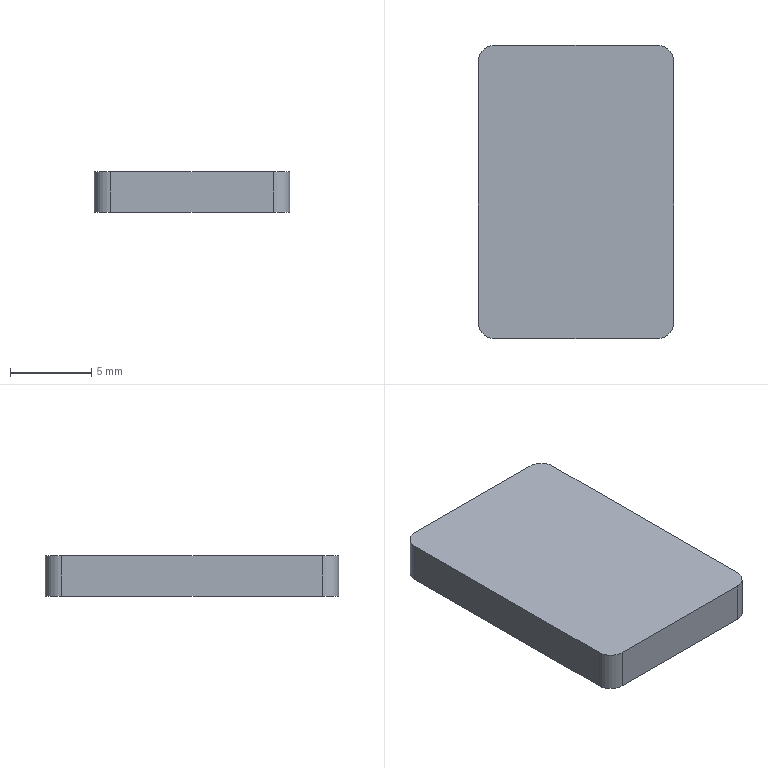Part | STEP file | lll_id938_x_t | 1 solid | 10 faces | box 12 x 18 x 2.5 mm | volume 537.854 mm3 | plane 6 | cylinder 4 | commonest cylinder face diameters 2 x4
STEP:
#1=CARTESIAN_POINT('',(498.87,-355.5,0.));
#2=VERTEX_POINT('',#1);
#3=CARTESIAN_POINT('',(498.87,-339.5,0.));
#4=VERTEX_POINT('',#3);
#5=CARTESIAN_POINT('',(498.87,-355.5,0.));
#6=DIRECTION('',(0.,1.,0.));
#7=VECTOR('',#6,1.);
#8=LINE('',#5,#7);
#9=EDGE_CURVE('',#2,#4,#8,.T.);
#10=ORIENTED_EDGE('',*,*,#9,.T.);
#11=CARTESIAN_POINT('',(498.87,-339.5,2.5));
#12=VERTEX_POINT('',#11);
#13=CARTESIAN_POINT('',(498.87,-339.5,2.5));
#14=DIRECTION('',(0.,0.,-1.));
#15=VECTOR('',#14,1.);
#16=LINE('',#13,#15);
#17=EDGE_CURVE('',#12,#4,#16,.T.);
#18=ORIENTED_EDGE('',*,*,#17,.F.);
#19=CARTESIAN_POINT('',(498.87,-355.5,2.5));
#20=VERTEX_POINT('',#19);
#21=CARTESIAN_POINT('',(498.87,-355.5,2.5));
#22=DIRECTION('',(0.,1.,0.));
#23=VECTOR('',#22,1.);
#24=LINE('',#21,#23);
#25=EDGE_CURVE('',#20,#12,#24,.T.);
#26=ORIENTED_EDGE('',*,*,#25,.F.);
#27=CARTESIAN_POINT('',(498.87,-355.5,2.5));
#28=DIRECTION('',(0.,0.,-1.));
#29=VECTOR('',#28,1.);
#30=LINE('',#27,#29);
#31=EDGE_CURVE('',#20,#2,#30,.T.);
#32=ORIENTED_EDGE('',*,*,#31,.T.);
#33=EDGE_LOOP('',(#10,#18,#26,#32));
#34=FACE_OUTER_BOUND('',#33,.T.);
#35=CARTESIAN_POINT('',(498.87,-355.5,2.5));
#36=DIRECTION('',(1.,0.,0.));
#37=DIRECTION('',(0.,0.,-1.));
#38=AXIS2_PLACEMENT_3D('',#35,#36,#37);
#39=PLANE('',#38);
#40=ADVANCED_FACE('',(#34),#39,.T.);
#41=CARTESIAN_POINT('',(497.87,-338.5,0.));
#42=VERTEX_POINT('',#41);
#43=CARTESIAN_POINT('',(497.87,-339.5,0.));
#44=DIRECTION('',(0.,0.,1.));
#45=DIRECTION('',(-1.,0.,0.));
#46=AXIS2_PLACEMENT_3D('',#43,#44,#45);
#47=CIRCLE('',#46,1.);
#48=EDGE_CURVE('',#4,#42,#47,.T.);
#49=ORIENTED_EDGE('',*,*,#48,.T.);
#50=CARTESIAN_POINT('',(497.87,-338.5,2.5));
#51=VERTEX_POINT('',#50);
#52=CARTESIAN_POINT('',(497.87,-338.5,2.5));
#53=DIRECTION('',(0.,0.,-1.));
#54=VECTOR('',#53,1.);
#55=LINE('',#52,#54);
#56=EDGE_CURVE('',#51,#42,#55,.T.);
#57=ORIENTED_EDGE('',*,*,#56,.F.);
#58=CARTESIAN_POINT('',(497.87,-339.5,2.5));
#59=DIRECTION('',(0.,0.,1.));
#60=DIRECTION('',(-1.,0.,0.));
#61=AXIS2_PLACEMENT_3D('',#58,#59,#60);
#62=CIRCLE('',#61,1.);
#63=EDGE_CURVE('',#12,#51,#62,.T.);
#64=ORIENTED_EDGE('',*,*,#63,.F.);
#65=ORIENTED_EDGE('',*,*,#17,.T.);
#66=EDGE_LOOP('',(#49,#57,#64,#65));
#67=FACE_OUTER_BOUND('',#66,.T.);
#68=CARTESIAN_POINT('',(497.87,-339.5,2.5));
#69=DIRECTION('',(0.,0.,-1.));
#70=DIRECTION('',(-1.,0.,0.));
#71=AXIS2_PLACEMENT_3D('',#68,#69,#70);
#72=CYLINDRICAL_SURFACE('',#71,1.);
#73=ADVANCED_FACE('',(#67),#72,.T.);
#74=CARTESIAN_POINT('',(487.87,-338.5,0.));
#75=VERTEX_POINT('',#74);
#76=CARTESIAN_POINT('',(497.87,-338.5,0.));
#77=DIRECTION('',(-1.,0.,0.));
#78=VECTOR('',#77,1.);
#79=LINE('',#76,#78);
#80=EDGE_CURVE('',#42,#75,#79,.T.);
#81=ORIENTED_EDGE('',*,*,#80,.T.);
#82=CARTESIAN_POINT('',(487.87,-338.5,2.5));
#83=VERTEX_POINT('',#82);
#84=CARTESIAN_POINT('',(487.87,-338.5,2.5));
#85=DIRECTION('',(0.,0.,-1.));
#86=VECTOR('',#85,1.);
#87=LINE('',#84,#86);
#88=EDGE_CURVE('',#83,#75,#87,.T.);
#89=ORIENTED_EDGE('',*,*,#88,.F.);
#90=CARTESIAN_POINT('',(497.87,-338.5,2.5));
#91=DIRECTION('',(-1.,0.,0.));
#92=VECTOR('',#91,1.);
#93=LINE('',#90,#92);
#94=EDGE_CURVE('',#51,#83,#93,.T.);
#95=ORIENTED_EDGE('',*,*,#94,.F.);
#96=ORIENTED_EDGE('',*,*,#56,.T.);
#97=EDGE_LOOP('',(#81,#89,#95,#96));
#98=FACE_OUTER_BOUND('',#97,.T.);
#99=CARTESIAN_POINT('',(497.87,-338.5,2.5));
#100=DIRECTION('',(0.,1.,0.));
#101=DIRECTION('',(0.,0.,-1.));
#102=AXIS2_PLACEMENT_3D('',#99,#100,#101);
#103=PLANE('',#102);
#104=ADVANCED_FACE('',(#98),#103,.T.);
#105=CARTESIAN_POINT('',(486.87,-339.5,0.));
#106=VERTEX_POINT('',#105);
#107=CARTESIAN_POINT('',(487.87,-339.5,0.));
#108=DIRECTION('',(0.,0.,1.));
#109=DIRECTION('',(-1.,0.,0.));
#110=AXIS2_PLACEMENT_3D('',#107,#108,#109);
#111=CIRCLE('',#110,1.);
#112=EDGE_CURVE('',#75,#106,#111,.T.);
#113=ORIENTED_EDGE('',*,*,#112,.T.);
#114=CARTESIAN_POINT('',(486.87,-339.5,2.5));
#115=VERTEX_POINT('',#114);
#116=CARTESIAN_POINT('',(486.87,-339.5,2.5));
#117=DIRECTION('',(0.,0.,-1.));
#118=VECTOR('',#117,1.);
#119=LINE('',#116,#118);
#120=EDGE_CURVE('',#115,#106,#119,.T.);
#121=ORIENTED_EDGE('',*,*,#120,.F.);
#122=CARTESIAN_POINT('',(487.87,-339.5,2.5));
#123=DIRECTION('',(0.,0.,1.));
#124=DIRECTION('',(-1.,0.,0.));
#125=AXIS2_PLACEMENT_3D('',#122,#123,#124);
#126=CIRCLE('',#125,1.);
#127=EDGE_CURVE('',#83,#115,#126,.T.);
#128=ORIENTED_EDGE('',*,*,#127,.F.);
#129=ORIENTED_EDGE('',*,*,#88,.T.);
#130=EDGE_LOOP('',(#113,#121,#128,#129));
#131=FACE_OUTER_BOUND('',#130,.T.);
#132=CARTESIAN_POINT('',(487.87,-339.5,2.5));
#133=DIRECTION('',(0.,0.,-1.));
#134=DIRECTION('',(-1.,0.,0.));
#135=AXIS2_PLACEMENT_3D('',#132,#133,#134);
#136=CYLINDRICAL_SURFACE('',#135,1.);
#137=ADVANCED_FACE('',(#131),#136,.T.);
#138=CARTESIAN_POINT('',(486.87,-355.5,0.));
#139=VERTEX_POINT('',#138);
#140=CARTESIAN_POINT('',(486.87,-339.5,0.));
#141=DIRECTION('',(0.,-1.,0.));
#142=VECTOR('',#141,1.);
#143=LINE('',#140,#142);
#144=EDGE_CURVE('',#106,#139,#143,.T.);
#145=ORIENTED_EDGE('',*,*,#144,.T.);
#146=CARTESIAN_POINT('',(486.87,-355.5,2.5));
#147=VERTEX_POINT('',#146);
#148=CARTESIAN_POINT('',(486.87,-355.5,2.5));
#149=DIRECTION('',(0.,0.,-1.));
#150=VECTOR('',#149,1.);
#151=LINE('',#148,#150);
#152=EDGE_CURVE('',#147,#139,#151,.T.);
#153=ORIENTED_EDGE('',*,*,#152,.F.);
#154=CARTESIAN_POINT('',(486.87,-339.5,2.5));
#155=DIRECTION('',(0.,-1.,0.));
#156=VECTOR('',#155,1.);
#157=LINE('',#154,#156);
#158=EDGE_CURVE('',#115,#147,#157,.T.);
#159=ORIENTED_EDGE('',*,*,#158,.F.);
#160=ORIENTED_EDGE('',*,*,#120,.T.);
#161=EDGE_LOOP('',(#145,#153,#159,#160));
#162=FACE_OUTER_BOUND('',#161,.T.);
#163=CARTESIAN_POINT('',(486.87,-339.5,2.5));
#164=DIRECTION('',(-1.,0.,0.));
#165=DIRECTION('',(0.,0.,1.));
#166=AXIS2_PLACEMENT_3D('',#163,#164,#165);
#167=PLANE('',#166);
#168=ADVANCED_FACE('',(#162),#167,.T.);
#169=CARTESIAN_POINT('',(487.87,-356.5,0.));
#170=VERTEX_POINT('',#169);
#171=CARTESIAN_POINT('',(487.87,-355.5,0.));
#172=DIRECTION('',(0.,0.,1.));
#173=DIRECTION('',(-1.,0.,0.));
#174=AXIS2_PLACEMENT_3D('',#171,#172,#173);
#175=CIRCLE('',#174,1.);
#176=EDGE_CURVE('',#139,#170,#175,.T.);
#177=ORIENTED_EDGE('',*,*,#176,.T.);
#178=CARTESIAN_POINT('',(487.87,-356.5,2.5));
#179=VERTEX_POINT('',#178);
#180=CARTESIAN_POINT('',(487.87,-356.5,2.5));
#181=DIRECTION('',(0.,0.,-1.));
#182=VECTOR('',#181,1.);
#183=LINE('',#180,#182);
#184=EDGE_CURVE('',#179,#170,#183,.T.);
#185=ORIENTED_EDGE('',*,*,#184,.F.);
#186=CARTESIAN_POINT('',(487.87,-355.5,2.5));
#187=DIRECTION('',(0.,0.,1.));
#188=DIRECTION('',(-1.,0.,0.));
#189=AXIS2_PLACEMENT_3D('',#186,#187,#188);
#190=CIRCLE('',#189,1.);
#191=EDGE_CURVE('',#147,#179,#190,.T.);
#192=ORIENTED_EDGE('',*,*,#191,.F.);
#193=ORIENTED_EDGE('',*,*,#152,.T.);
#194=EDGE_LOOP('',(#177,#185,#192,#193));
#195=FACE_OUTER_BOUND('',#194,.T.);
#196=CARTESIAN_POINT('',(487.87,-355.5,2.5));
#197=DIRECTION('',(0.,0.,-1.));
#198=DIRECTION('',(-1.,0.,0.));
#199=AXIS2_PLACEMENT_3D('',#196,#197,#198);
#200=CYLINDRICAL_SURFACE('',#199,1.);
#201=ADVANCED_FACE('',(#195),#200,.T.);
#202=CARTESIAN_POINT('',(497.87,-356.5,0.));
#203=VERTEX_POINT('',#202);
#204=CARTESIAN_POINT('',(487.87,-356.5,0.));
#205=DIRECTION('',(1.,0.,0.));
#206=VECTOR('',#205,1.);
#207=LINE('',#204,#206);
#208=EDGE_CURVE('',#170,#203,#207,.T.);
#209=ORIENTED_EDGE('',*,*,#208,.T.);
#210=CARTESIAN_POINT('',(497.87,-356.5,2.5));
#211=VERTEX_POINT('',#210);
#212=CARTESIAN_POINT('',(497.87,-356.5,2.5));
#213=DIRECTION('',(0.,0.,-1.));
#214=VECTOR('',#213,1.);
#215=LINE('',#212,#214);
#216=EDGE_CURVE('',#211,#203,#215,.T.);
#217=ORIENTED_EDGE('',*,*,#216,.F.);
#218=CARTESIAN_POINT('',(487.87,-356.5,2.5));
#219=DIRECTION('',(1.,0.,0.));
#220=VECTOR('',#219,1.);
#221=LINE('',#218,#220);
#222=EDGE_CURVE('',#179,#211,#221,.T.);
#223=ORIENTED_EDGE('',*,*,#222,.F.);
#224=ORIENTED_EDGE('',*,*,#184,.T.);
#225=EDGE_LOOP('',(#209,#217,#223,#224));
#226=FACE_OUTER_BOUND('',#225,.T.);
#227=CARTESIAN_POINT('',(487.87,-356.5,2.5));
#228=DIRECTION('',(0.,-1.,0.));
#229=DIRECTION('',(0.,0.,1.));
#230=AXIS2_PLACEMENT_3D('',#227,#228,#229);
#231=PLANE('',#230);
#232=ADVANCED_FACE('',(#226),#231,.T.);
#233=CARTESIAN_POINT('',(497.87,-355.5,0.));
#234=DIRECTION('',(0.,0.,1.));
#235=DIRECTION('',(-1.,0.,0.));
#236=AXIS2_PLACEMENT_3D('',#233,#234,#235);
#237=CIRCLE('',#236,1.);
#238=EDGE_CURVE('',#203,#2,#237,.T.);
#239=ORIENTED_EDGE('',*,*,#238,.T.);
#240=ORIENTED_EDGE('',*,*,#31,.F.);
#241=CARTESIAN_POINT('',(497.87,-355.5,2.5));
#242=DIRECTION('',(0.,0.,1.));
#243=DIRECTION('',(-1.,0.,0.));
#244=AXIS2_PLACEMENT_3D('',#241,#242,#243);
#245=CIRCLE('',#244,1.);
#246=EDGE_CURVE('',#211,#20,#245,.T.);
#247=ORIENTED_EDGE('',*,*,#246,.F.);
#248=ORIENTED_EDGE('',*,*,#216,.T.);
#249=EDGE_LOOP('',(#239,#240,#247,#248));
#250=FACE_OUTER_BOUND('',#249,.T.);
#251=CARTESIAN_POINT('',(497.87,-355.5,2.5));
#252=DIRECTION('',(0.,0.,-1.));
#253=DIRECTION('',(-1.,0.,0.));
#254=AXIS2_PLACEMENT_3D('',#251,#252,#253);
#255=CYLINDRICAL_SURFACE('',#254,1.);
#256=ADVANCED_FACE('',(#250),#255,.T.);
#257=ORIENTED_EDGE('',*,*,#25,.T.);
#258=ORIENTED_EDGE('',*,*,#63,.T.);
#259=ORIENTED_EDGE('',*,*,#94,.T.);
#260=ORIENTED_EDGE('',*,*,#127,.T.);
#261=ORIENTED_EDGE('',*,*,#158,.T.);
#262=ORIENTED_EDGE('',*,*,#191,.T.);
#263=ORIENTED_EDGE('',*,*,#222,.T.);
#264=ORIENTED_EDGE('',*,*,#246,.T.);
#265=EDGE_LOOP('',(#257,#258,#259,#260,#261,#262,#263,#264));
#266=FACE_OUTER_BOUND('',#265,.T.);
#267=CARTESIAN_POINT('',(497.87,-339.5,2.5));
#268=DIRECTION('',(0.,0.,-1.));
#269=DIRECTION('',(-1.,0.,0.));
#270=AXIS2_PLACEMENT_3D('',#267,#268,#269);
#271=PLANE('',#270);
#272=ADVANCED_FACE('',(#266),#271,.F.);
#273=ORIENTED_EDGE('',*,*,#9,.F.);
#274=ORIENTED_EDGE('',*,*,#238,.F.);
#275=ORIENTED_EDGE('',*,*,#208,.F.);
#276=ORIENTED_EDGE('',*,*,#176,.F.);
#277=ORIENTED_EDGE('',*,*,#144,.F.);
#278=ORIENTED_EDGE('',*,*,#112,.F.);
#279=ORIENTED_EDGE('',*,*,#80,.F.);
#280=ORIENTED_EDGE('',*,*,#48,.F.);
#281=EDGE_LOOP('',(#273,#274,#275,#276,#277,#278,#279,#280));
#282=FACE_OUTER_BOUND('',#281,.T.);
#283=CARTESIAN_POINT('',(497.87,-339.5,0.));
#284=DIRECTION('',(0.,0.,-1.));
#285=DIRECTION('',(-1.,0.,0.));
#286=AXIS2_PLACEMENT_3D('',#283,#284,#285);
#287=PLANE('',#286);
#288=ADVANCED_FACE('',(#282),#287,.T.);
#289=CLOSED_SHELL('',(#40,#73,#104,#137,#168,#201,#232,#256,#272,#288));
#290=MANIFOLD_SOLID_BREP('',#289);
#291=(LENGTH_UNIT()NAMED_UNIT(*)SI_UNIT(.MILLI.,.METRE.));
#292=UNCERTAINTY_MEASURE_WITH_UNIT(LENGTH_MEASURE(0.00002),#291,'','');
#293=(NAMED_UNIT(*)PLANE_ANGLE_UNIT()SI_UNIT($,.RADIAN.));
#294=PLANE_ANGLE_MEASURE_WITH_UNIT(PLANE_ANGLE_MEASURE(0.01745),#293);
#295=DIMENSIONAL_EXPONENTS(0.,0.,0.,0.,0.,0.,0.);
#296=(CONVERSION_BASED_UNIT('DEGREE',#294)NAMED_UNIT(#295)PLANE_ANGLE_UNIT());
#297=(NAMED_UNIT(*)SI_UNIT($,.STERADIAN.)SOLID_ANGLE_UNIT());
#298=(GEOMETRIC_REPRESENTATION_CONTEXT(3)GLOBAL_UNCERTAINTY_ASSIGNED_CONTEXT((#292))GLOBAL_UNIT_ASSIGNED_CONTEXT((#291,#296,#297))REPRESENTATION_CONTEXT('',''));
#299=ADVANCED_BREP_SHAPE_REPRESENTATION('',(#290),#298);